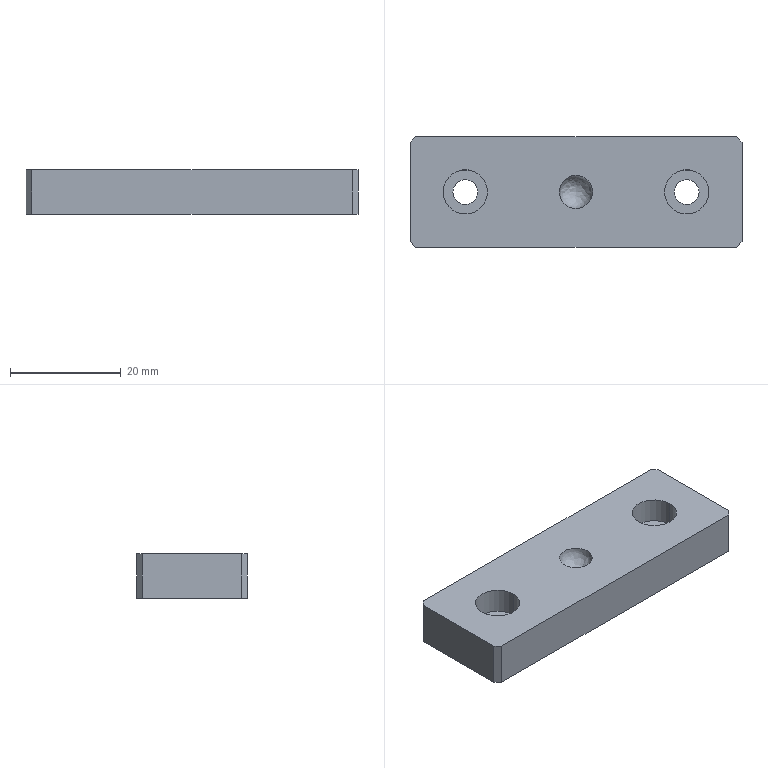Part | STEP file | Displacement press plate | 1 solid | 21 faces | box 60 x 20 x 8 mm | volume 8957 mm3 | plane 12 | cylinder 8 | spline 1 | commonest cylinder face diameters 4.5 x4 8 x4